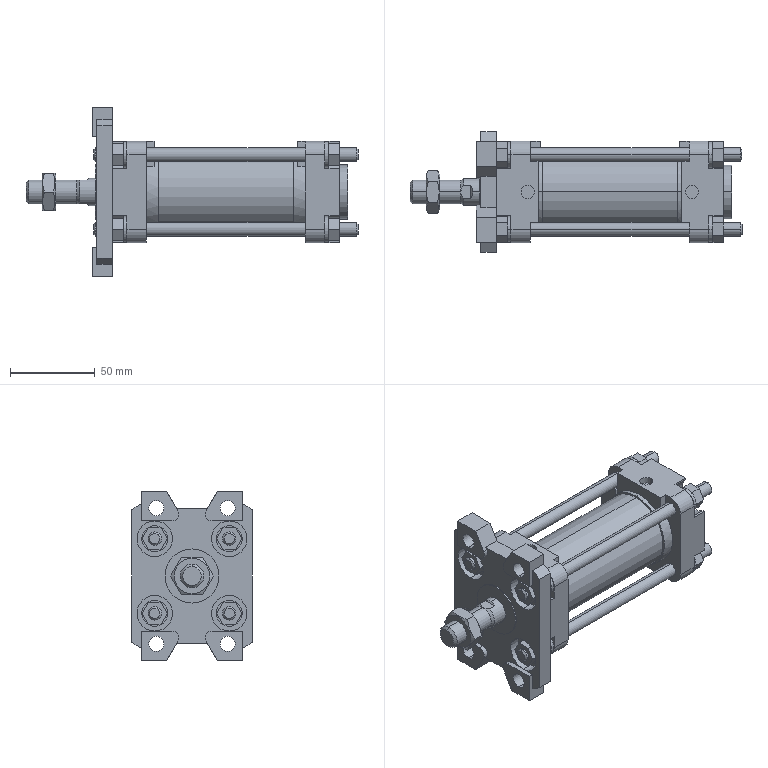Part | STEP file | CA2F40-50Z_0_0_0_ | 4 solids | 379 faces | box 196 x 71 x 100 mm | volume 325906 mm3 | plane 215 | cylinder 128 | cone 36 | commonest cylinder face diameters 8 x36 15.4 x24 21 x20 16 x12 9 x8 32 x6